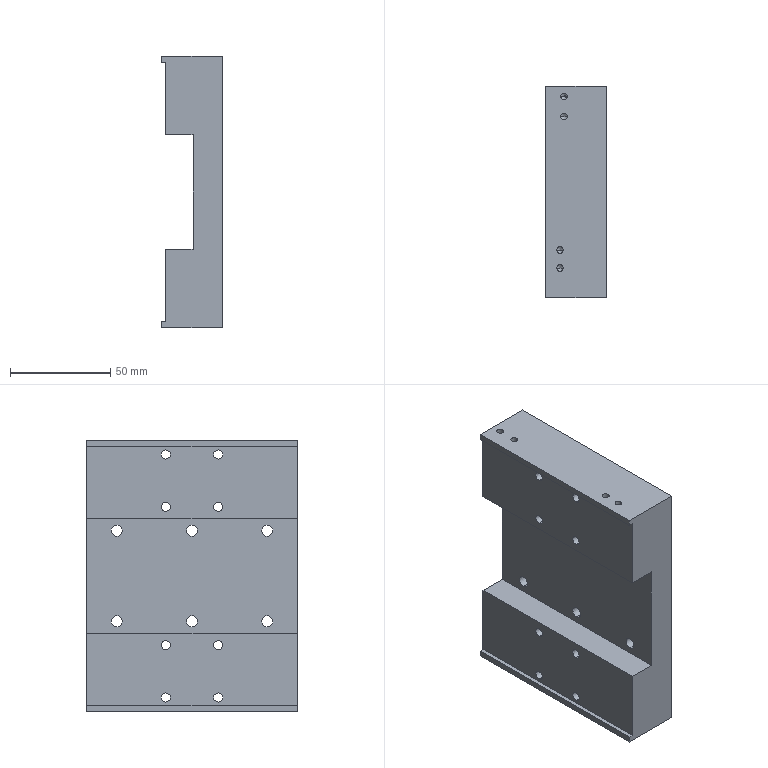Part | SolidWorks | features HoleWzd 9, ICE 2, Extrusion 1, MirrorPattern 1 | 1 solid | 140 faces | box 30 x 105 x 135 mm | volume 301604 mm3 | cylinder 84 | cone 28 | plane 28 | commonest cylinder face diameters 3.3 x16 4.5 x16 8 x16 5.5 x12 10 x12 5 x8